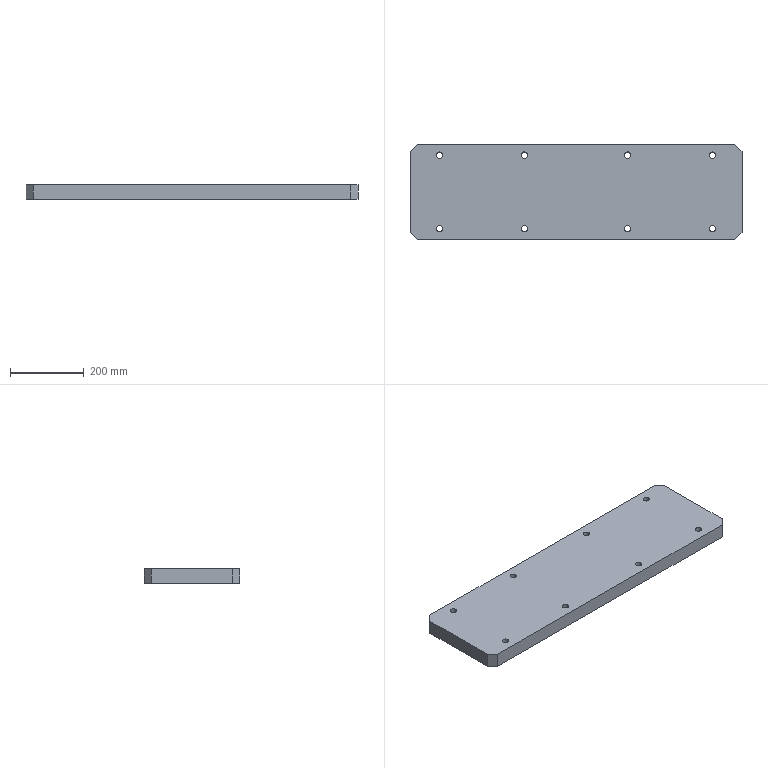Part | SolidWorks | features Chamfer 1, Extrusion 1, HoleWzd 1 | 1 solid | 26 faces | box 900 x 260 x 40 mm | volume 9255366 mm3 | cylinder 16 | plane 10 | commonest cylinder face diameters 17 x16
STEP:
#1=CARTESIAN_POINT('',(-378.5,100.,0.));
#2=VERTEX_POINT('',#1);
#3=CARTESIAN_POINT('',(-361.5,100.,0.));
#4=VERTEX_POINT('',#3);
#5=CARTESIAN_POINT('',(-370.,100.,0.));
#6=DIRECTION('',(0.,0.,1.));
#7=DIRECTION('',(1.,0.,0.));
#8=AXIS2_PLACEMENT_3D('',#5,#6,#7);
#9=CIRCLE('',#8,8.5);
#10=EDGE_CURVE('',#2,#4,#9,.T.);
#11=ORIENTED_EDGE('',*,*,#10,.F.);
#12=CARTESIAN_POINT('',(-378.5,100.,40.));
#13=VERTEX_POINT('',#12);
#14=CARTESIAN_POINT('',(-378.5,100.,40.));
#15=DIRECTION('',(0.,0.,1.));
#16=VECTOR('',#15,1000.);
#17=LINE('',#14,#16);
#18=EDGE_CURVE('',#2,#13,#17,.T.);
#19=ORIENTED_EDGE('',*,*,#18,.T.);
#20=CARTESIAN_POINT('',(-361.5,100.,40.));
#21=VERTEX_POINT('',#20);
#22=CARTESIAN_POINT('',(-370.,100.,40.));
#23=DIRECTION('',(0.,0.,1.));
#24=DIRECTION('',(1.,0.,0.));
#25=AXIS2_PLACEMENT_3D('',#22,#23,#24);
#26=CIRCLE('',#25,8.5);
#27=EDGE_CURVE('',#13,#21,#26,.T.);
#28=ORIENTED_EDGE('',*,*,#27,.T.);
#29=CARTESIAN_POINT('',(-361.5,100.,40.));
#30=DIRECTION('',(0.,0.,1.));
#31=VECTOR('',#30,1000.);
#32=LINE('',#29,#31);
#33=EDGE_CURVE('',#4,#21,#32,.T.);
#34=ORIENTED_EDGE('',*,*,#33,.F.);
#35=EDGE_LOOP('',(#11,#19,#28,#34));
#36=FACE_OUTER_BOUND('',#35,.T.);
#37=CARTESIAN_POINT('',(-370.,100.,40.));
#38=DIRECTION('',(0.,0.,1.));
#39=DIRECTION('',(1.,0.,0.));
#40=AXIS2_PLACEMENT_3D('',#37,#38,#39);
#41=CYLINDRICAL_SURFACE('',#40,8.5);
#42=ADVANCED_FACE('',(#36),#41,.F.);
#43=CARTESIAN_POINT('',(-148.5,100.,0.));
#44=VERTEX_POINT('',#43);
#45=CARTESIAN_POINT('',(-131.5,100.,0.));
#46=VERTEX_POINT('',#45);
#47=CARTESIAN_POINT('',(-140.,100.,0.));
#48=DIRECTION('',(0.,0.,1.));
#49=DIRECTION('',(1.,0.,0.));
#50=AXIS2_PLACEMENT_3D('',#47,#48,#49);
#51=CIRCLE('',#50,8.5);
#52=EDGE_CURVE('',#44,#46,#51,.T.);
#53=ORIENTED_EDGE('',*,*,#52,.F.);
#54=CARTESIAN_POINT('',(-148.5,100.,40.));
#55=VERTEX_POINT('',#54);
#56=CARTESIAN_POINT('',(-148.5,100.,40.));
#57=DIRECTION('',(0.,0.,1.));
#58=VECTOR('',#57,1000.);
#59=LINE('',#56,#58);
#60=EDGE_CURVE('',#44,#55,#59,.T.);
#61=ORIENTED_EDGE('',*,*,#60,.T.);
#62=CARTESIAN_POINT('',(-131.5,100.,40.));
#63=VERTEX_POINT('',#62);
#64=CARTESIAN_POINT('',(-140.,100.,40.));
#65=DIRECTION('',(0.,0.,1.));
#66=DIRECTION('',(1.,0.,0.));
#67=AXIS2_PLACEMENT_3D('',#64,#65,#66);
#68=CIRCLE('',#67,8.5);
#69=EDGE_CURVE('',#55,#63,#68,.T.);
#70=ORIENTED_EDGE('',*,*,#69,.T.);
#71=CARTESIAN_POINT('',(-131.5,100.,40.));
#72=DIRECTION('',(0.,0.,1.));
#73=VECTOR('',#72,1000.);
#74=LINE('',#71,#73);
#75=EDGE_CURVE('',#46,#63,#74,.T.);
#76=ORIENTED_EDGE('',*,*,#75,.F.);
#77=EDGE_LOOP('',(#53,#61,#70,#76));
#78=FACE_OUTER_BOUND('',#77,.T.);
#79=CARTESIAN_POINT('',(-140.,100.,40.));
#80=DIRECTION('',(0.,0.,1.));
#81=DIRECTION('',(1.,0.,0.));
#82=AXIS2_PLACEMENT_3D('',#79,#80,#81);
#83=CYLINDRICAL_SURFACE('',#82,8.5);
#84=ADVANCED_FACE('',(#78),#83,.F.);
#85=CARTESIAN_POINT('',(-378.5,-100.,0.));
#86=VERTEX_POINT('',#85);
#87=CARTESIAN_POINT('',(-361.5,-100.,0.));
#88=VERTEX_POINT('',#87);
#89=CARTESIAN_POINT('',(-370.,-100.,0.));
#90=DIRECTION('',(0.,0.,1.));
#91=DIRECTION('',(1.,0.,0.));
#92=AXIS2_PLACEMENT_3D('',#89,#90,#91);
#93=CIRCLE('',#92,8.5);
#94=EDGE_CURVE('',#86,#88,#93,.T.);
#95=ORIENTED_EDGE('',*,*,#94,.F.);
#96=CARTESIAN_POINT('',(-378.5,-100.,40.));
#97=VERTEX_POINT('',#96);
#98=CARTESIAN_POINT('',(-378.5,-100.,40.));
#99=DIRECTION('',(0.,0.,1.));
#100=VECTOR('',#99,1000.);
#101=LINE('',#98,#100);
#102=EDGE_CURVE('',#86,#97,#101,.T.);
#103=ORIENTED_EDGE('',*,*,#102,.T.);
#104=CARTESIAN_POINT('',(-361.5,-100.,40.));
#105=VERTEX_POINT('',#104);
#106=CARTESIAN_POINT('',(-370.,-100.,40.));
#107=DIRECTION('',(0.,0.,1.));
#108=DIRECTION('',(1.,0.,0.));
#109=AXIS2_PLACEMENT_3D('',#106,#107,#108);
#110=CIRCLE('',#109,8.5);
#111=EDGE_CURVE('',#97,#105,#110,.T.);
#112=ORIENTED_EDGE('',*,*,#111,.T.);
#113=CARTESIAN_POINT('',(-361.5,-100.,40.));
#114=DIRECTION('',(0.,0.,1.));
#115=VECTOR('',#114,1000.);
#116=LINE('',#113,#115);
#117=EDGE_CURVE('',#88,#105,#116,.T.);
#118=ORIENTED_EDGE('',*,*,#117,.F.);
#119=EDGE_LOOP('',(#95,#103,#112,#118));
#120=FACE_OUTER_BOUND('',#119,.T.);
#121=CARTESIAN_POINT('',(-370.,-100.,40.));
#122=DIRECTION('',(0.,0.,1.));
#123=DIRECTION('',(1.,0.,0.));
#124=AXIS2_PLACEMENT_3D('',#121,#122,#123);
#125=CYLINDRICAL_SURFACE('',#124,8.5);
#126=ADVANCED_FACE('',(#120),#125,.F.);
#127=CARTESIAN_POINT('',(-148.5,-100.,0.));
#128=VERTEX_POINT('',#127);
#129=CARTESIAN_POINT('',(-131.5,-100.,0.));
#130=VERTEX_POINT('',#129);
#131=CARTESIAN_POINT('',(-140.,-100.,0.));
#132=DIRECTION('',(0.,0.,1.));
#133=DIRECTION('',(1.,0.,0.));
#134=AXIS2_PLACEMENT_3D('',#131,#132,#133);
#135=CIRCLE('',#134,8.5);
#136=EDGE_CURVE('',#128,#130,#135,.T.);
#137=ORIENTED_EDGE('',*,*,#136,.F.);
#138=CARTESIAN_POINT('',(-148.5,-100.,40.));
#139=VERTEX_POINT('',#138);
#140=CARTESIAN_POINT('',(-148.5,-100.,40.));
#141=DIRECTION('',(0.,0.,1.));
#142=VECTOR('',#141,1000.);
#143=LINE('',#140,#142);
#144=EDGE_CURVE('',#128,#139,#143,.T.);
#145=ORIENTED_EDGE('',*,*,#144,.T.);
#146=CARTESIAN_POINT('',(-131.5,-100.,40.));
#147=VERTEX_POINT('',#146);
#148=CARTESIAN_POINT('',(-140.,-100.,40.));
#149=DIRECTION('',(0.,0.,1.));
#150=DIRECTION('',(1.,0.,0.));
#151=AXIS2_PLACEMENT_3D('',#148,#149,#150);
#152=CIRCLE('',#151,8.5);
#153=EDGE_CURVE('',#139,#147,#152,.T.);
#154=ORIENTED_EDGE('',*,*,#153,.T.);
#155=CARTESIAN_POINT('',(-131.5,-100.,40.));
#156=DIRECTION('',(0.,0.,1.));
#157=VECTOR('',#156,1000.);
#158=LINE('',#155,#157);
#159=EDGE_CURVE('',#130,#147,#158,.T.);
#160=ORIENTED_EDGE('',*,*,#159,.F.);
#161=EDGE_LOOP('',(#137,#145,#154,#160));
#162=FACE_OUTER_BOUND('',#161,.T.);
#163=CARTESIAN_POINT('',(-140.,-100.,40.));
#164=DIRECTION('',(0.,0.,1.));
#165=DIRECTION('',(1.,0.,0.));
#166=AXIS2_PLACEMENT_3D('',#163,#164,#165);
#167=CYLINDRICAL_SURFACE('',#166,8.5);
#168=ADVANCED_FACE('',(#162),#167,.F.);
#169=CARTESIAN_POINT('',(131.5,-100.,0.));
#170=VERTEX_POINT('',#169);
#171=CARTESIAN_POINT('',(148.5,-100.,0.));
#172=VERTEX_POINT('',#171);
#173=CARTESIAN_POINT('',(140.,-100.,0.));
#174=DIRECTION('',(0.,0.,1.));
#175=DIRECTION('',(1.,0.,0.));
#176=AXIS2_PLACEMENT_3D('',#173,#174,#175);
#177=CIRCLE('',#176,8.5);
#178=EDGE_CURVE('',#170,#172,#177,.T.);
#179=ORIENTED_EDGE('',*,*,#178,.F.);
#180=CARTESIAN_POINT('',(131.5,-100.,40.));
#181=VERTEX_POINT('',#180);
#182=CARTESIAN_POINT('',(131.5,-100.,40.));
#183=DIRECTION('',(0.,0.,1.));
#184=VECTOR('',#183,1000.);
#185=LINE('',#182,#184);
#186=EDGE_CURVE('',#170,#181,#185,.T.);
#187=ORIENTED_EDGE('',*,*,#186,.T.);
#188=CARTESIAN_POINT('',(148.5,-100.,40.));
#189=VERTEX_POINT('',#188);
#190=CARTESIAN_POINT('',(140.,-100.,40.));
#191=DIRECTION('',(0.,0.,1.));
#192=DIRECTION('',(1.,0.,0.));
#193=AXIS2_PLACEMENT_3D('',#190,#191,#192);
#194=CIRCLE('',#193,8.5);
#195=EDGE_CURVE('',#181,#189,#194,.T.);
#196=ORIENTED_EDGE('',*,*,#195,.T.);
#197=CARTESIAN_POINT('',(148.5,-100.,40.));
#198=DIRECTION('',(0.,0.,1.));
#199=VECTOR('',#198,1000.);
#200=LINE('',#197,#199);
#201=EDGE_CURVE('',#172,#189,#200,.T.);
#202=ORIENTED_EDGE('',*,*,#201,.F.);
#203=EDGE_LOOP('',(#179,#187,#196,#202));
#204=FACE_OUTER_BOUND('',#203,.T.);
#205=CARTESIAN_POINT('',(140.,-100.,40.));
#206=DIRECTION('',(0.,0.,1.));
#207=DIRECTION('',(1.,0.,0.));
#208=AXIS2_PLACEMENT_3D('',#205,#206,#207);
#209=CYLINDRICAL_SURFACE('',#208,8.5);
#210=ADVANCED_FACE('',(#204),#209,.F.);
#211=CARTESIAN_POINT('',(361.5,-100.,0.));
#212=VERTEX_POINT('',#211);
#213=CARTESIAN_POINT('',(378.5,-100.,0.));
#214=VERTEX_POINT('',#213);
#215=CARTESIAN_POINT('',(370.,-100.,0.));
#216=DIRECTION('',(0.,0.,1.));
#217=DIRECTION('',(1.,0.,0.));
#218=AXIS2_PLACEMENT_3D('',#215,#216,#217);
#219=CIRCLE('',#218,8.5);
#220=EDGE_CURVE('',#212,#214,#219,.T.);
#221=ORIENTED_EDGE('',*,*,#220,.F.);
#222=CARTESIAN_POINT('',(361.5,-100.,40.));
#223=VERTEX_POINT('',#222);
#224=CARTESIAN_POINT('',(361.5,-100.,40.));
#225=DIRECTION('',(0.,0.,1.));
#226=VECTOR('',#225,1000.);
#227=LINE('',#224,#226);
#228=EDGE_CURVE('',#212,#223,#227,.T.);
#229=ORIENTED_EDGE('',*,*,#228,.T.);
#230=CARTESIAN_POINT('',(378.5,-100.,40.));
#231=VERTEX_POINT('',#230);
#232=CARTESIAN_POINT('',(370.,-100.,40.));
#233=DIRECTION('',(0.,0.,1.));
#234=DIRECTION('',(1.,0.,0.));
#235=AXIS2_PLACEMENT_3D('',#232,#233,#234);
#236=CIRCLE('',#235,8.5);
#237=EDGE_CURVE('',#223,#231,#236,.T.);
#238=ORIENTED_EDGE('',*,*,#237,.T.);
#239=CARTESIAN_POINT('',(378.5,-100.,40.));
#240=DIRECTION('',(0.,0.,1.));
#241=VECTOR('',#240,1000.);
#242=LINE('',#239,#241);
#243=EDGE_CURVE('',#214,#231,#242,.T.);
#244=ORIENTED_EDGE('',*,*,#243,.F.);
#245=EDGE_LOOP('',(#221,#229,#238,#244));
#246=FACE_OUTER_BOUND('',#245,.T.);
#247=CARTESIAN_POINT('',(370.,-100.,40.));
#248=DIRECTION('',(0.,0.,1.));
#249=DIRECTION('',(1.,0.,0.));
#250=AXIS2_PLACEMENT_3D('',#247,#248,#249);
#251=CYLINDRICAL_SURFACE('',#250,8.5);
#252=ADVANCED_FACE('',(#246),#251,.F.);
#253=CARTESIAN_POINT('',(131.5,100.,0.));
#254=VERTEX_POINT('',#253);
#255=CARTESIAN_POINT('',(148.5,100.,0.));
#256=VERTEX_POINT('',#255);
#257=CARTESIAN_POINT('',(140.,100.,0.));
#258=DIRECTION('',(0.,0.,1.));
#259=DIRECTION('',(1.,0.,0.));
#260=AXIS2_PLACEMENT_3D('',#257,#258,#259);
#261=CIRCLE('',#260,8.5);
#262=EDGE_CURVE('',#254,#256,#261,.T.);
#263=ORIENTED_EDGE('',*,*,#262,.F.);
#264=CARTESIAN_POINT('',(131.5,100.,40.));
#265=VERTEX_POINT('',#264);
#266=CARTESIAN_POINT('',(131.5,100.,40.));
#267=DIRECTION('',(0.,0.,1.));
#268=VECTOR('',#267,1000.);
#269=LINE('',#266,#268);
#270=EDGE_CURVE('',#254,#265,#269,.T.);
#271=ORIENTED_EDGE('',*,*,#270,.T.);
#272=CARTESIAN_POINT('',(148.5,100.,40.));
#273=VERTEX_POINT('',#272);
#274=CARTESIAN_POINT('',(140.,100.,40.));
#275=DIRECTION('',(0.,0.,1.));
#276=DIRECTION('',(1.,0.,0.));
#277=AXIS2_PLACEMENT_3D('',#274,#275,#276);
#278=CIRCLE('',#277,8.5);
#279=EDGE_CURVE('',#265,#273,#278,.T.);
#280=ORIENTED_EDGE('',*,*,#279,.T.);
#281=CARTESIAN_POINT('',(148.5,100.,40.));
#282=DIRECTION('',(0.,0.,1.));
#283=VECTOR('',#282,1000.);
#284=LINE('',#281,#283);
#285=EDGE_CURVE('',#256,#273,#284,.T.);
#286=ORIENTED_EDGE('',*,*,#285,.F.);
#287=EDGE_LOOP('',(#263,#271,#280,#286));
#288=FACE_OUTER_BOUND('',#287,.T.);
#289=CARTESIAN_POINT('',(140.,100.,40.));
#290=DIRECTION('',(0.,0.,1.));
#291=DIRECTION('',(1.,0.,0.));
#292=AXIS2_PLACEMENT_3D('',#289,#290,#291);
#293=CYLINDRICAL_SURFACE('',#292,8.5);
#294=ADVANCED_FACE('',(#288),#293,.F.);
#295=CARTESIAN_POINT('',(361.5,100.,0.));
#296=VERTEX_POINT('',#295);
#297=CARTESIAN_POINT('',(378.5,100.,0.));
#298=VERTEX_POINT('',#297);
#299=CARTESIAN_POINT('',(370.,100.,0.));
#300=DIRECTION('',(0.,0.,1.));
#301=DIRECTION('',(1.,0.,0.));
#302=AXIS2_PLACEMENT_3D('',#299,#300,#301);
#303=CIRCLE('',#302,8.5);
#304=EDGE_CURVE('',#296,#298,#303,.T.);
#305=ORIENTED_EDGE('',*,*,#304,.F.);
#306=CARTESIAN_POINT('',(361.5,100.,40.));
#307=VERTEX_POINT('',#306);
#308=CARTESIAN_POINT('',(361.5,100.,40.));
#309=DIRECTION('',(0.,0.,1.));
#310=VECTOR('',#309,1000.);
#311=LINE('',#308,#310);
#312=EDGE_CURVE('',#296,#307,#311,.T.);
#313=ORIENTED_EDGE('',*,*,#312,.T.);
#314=CARTESIAN_POINT('',(378.5,100.,40.));
#315=VERTEX_POINT('',#314);
#316=CARTESIAN_POINT('',(370.,100.,40.));
#317=DIRECTION('',(0.,0.,1.));
#318=DIRECTION('',(1.,0.,0.));
#319=AXIS2_PLACEMENT_3D('',#316,#317,#318);
#320=CIRCLE('',#319,8.5);
#321=EDGE_CURVE('',#307,#315,#320,.T.);
#322=ORIENTED_EDGE('',*,*,#321,.T.);
#323=CARTESIAN_POINT('',(378.5,100.,40.));
#324=DIRECTION('',(0.,0.,1.));
#325=VECTOR('',#324,1000.);
#326=LINE('',#323,#325);
#327=EDGE_CURVE('',#298,#315,#326,.T.);
#328=ORIENTED_EDGE('',*,*,#327,.F.);
#329=EDGE_LOOP('',(#305,#313,#322,#328));
#330=FACE_OUTER_BOUND('',#329,.T.);
#331=CARTESIAN_POINT('',(370.,100.,40.));
#332=DIRECTION('',(0.,0.,1.));
#333=DIRECTION('',(1.,0.,0.));
#334=AXIS2_PLACEMENT_3D('',#331,#332,#333);
#335=CYLINDRICAL_SURFACE('',#334,8.5);
#336=ADVANCED_FACE('',(#330),#335,.F.);
#337=CARTESIAN_POINT('',(-450.,110.,40.));
#338=VERTEX_POINT('',#337);
#339=CARTESIAN_POINT('',(-450.,-110.,40.));
#340=VERTEX_POINT('',#339);
#341=CARTESIAN_POINT('',(-450.,-130.,40.));
#342=DIRECTION('',(0.,-1.,0.));
#343=VECTOR('',#342,1000.);
#344=LINE('',#341,#343);
#345=EDGE_CURVE('',#338,#340,#344,.T.);
#346=ORIENTED_EDGE('',*,*,#345,.F.);
#347=CARTESIAN_POINT('',(-450.,110.,0.));
#348=VERTEX_POINT('',#347);
#349=CARTESIAN_POINT('',(-450.,110.,40.));
#350=DIRECTION('',(0.,0.,-1.));
#351=VECTOR('',#350,1000.);
#352=LINE('',#349,#351);
#353=EDGE_CURVE('',#338,#348,#352,.T.);
#354=ORIENTED_EDGE('',*,*,#353,.T.);
#355=CARTESIAN_POINT('',(-450.,-110.,0.));
#356=VERTEX_POINT('',#355);
#357=CARTESIAN_POINT('',(-450.,-130.,0.));
#358=DIRECTION('',(0.,-1.,0.));
#359=VECTOR('',#358,1000.);
#360=LINE('',#357,#359);
#361=EDGE_CURVE('',#348,#356,#360,.T.);
#362=ORIENTED_EDGE('',*,*,#361,.T.);
#363=CARTESIAN_POINT('',(-450.,-110.,40.));
#364=DIRECTION('',(0.,0.,1.));
#365=VECTOR('',#364,1000.);
#366=LINE('',#363,#365);
#367=EDGE_CURVE('',#356,#340,#366,.T.);
#368=ORIENTED_EDGE('',*,*,#367,.T.);
#369=EDGE_LOOP('',(#346,#354,#362,#368));
#370=FACE_OUTER_BOUND('',#369,.T.);
#371=CARTESIAN_POINT('',(-450.,-130.,40.));
#372=DIRECTION('',(1.,0.,0.));
#373=DIRECTION('',(0.,0.,-1.));
#374=AXIS2_PLACEMENT_3D('',#371,#372,#373);
#375=PLANE('',#374);
#376=ADVANCED_FACE('',(#370),#375,.F.);
#377=CARTESIAN_POINT('',(-430.,-130.,0.));
#378=VERTEX_POINT('',#377);
#379=CARTESIAN_POINT('',(430.,-130.,0.));
#380=VERTEX_POINT('',#379);
#381=CARTESIAN_POINT('',(450.,-130.,0.));
#382=DIRECTION('',(1.,0.,0.));
#383=VECTOR('',#382,1000.);
#384=LINE('',#381,#383);
#385=EDGE_CURVE('',#378,#380,#384,.T.);
#386=ORIENTED_EDGE('',*,*,#385,.T.);
#387=CARTESIAN_POINT('',(430.,-130.,40.));
#388=VERTEX_POINT('',#387);
#389=CARTESIAN_POINT('',(430.,-130.,40.));
#390=DIRECTION('',(0.,0.,1.));
#391=VECTOR('',#390,1000.);
#392=LINE('',#389,#391);
#393=EDGE_CURVE('',#380,#388,#392,.T.);
#394=ORIENTED_EDGE('',*,*,#393,.T.);
#395=CARTESIAN_POINT('',(-430.,-130.,40.));
#396=VERTEX_POINT('',#395);
#397=CARTESIAN_POINT('',(450.,-130.,40.));
#398=DIRECTION('',(1.,0.,0.));
#399=VECTOR('',#398,1000.);
#400=LINE('',#397,#399);
#401=EDGE_CURVE('',#396,#388,#400,.T.);
#402=ORIENTED_EDGE('',*,*,#401,.F.);
#403=CARTESIAN_POINT('',(-430.,-130.,40.));
#404=DIRECTION('',(0.,0.,-1.));
#405=VECTOR('',#404,1000.);
#406=LINE('',#403,#405);
#407=EDGE_CURVE('',#396,#378,#406,.T.);
#408=ORIENTED_EDGE('',*,*,#407,.T.);
#409=EDGE_LOOP('',(#386,#394,#402,#408));
#410=FACE_OUTER_BOUND('',#409,.T.);
#411=CARTESIAN_POINT('',(450.,-130.,40.));
#412=DIRECTION('',(0.,1.,0.));
#413=DIRECTION('',(-1.,0.,0.));
#414=AXIS2_PLACEMENT_3D('',#411,#412,#413);
#415=PLANE('',#414);
#416=ADVANCED_FACE('',(#410),#415,.F.);
#417=CARTESIAN_POINT('',(450.,-110.,0.));
#418=VERTEX_POINT('',#417);
#419=CARTESIAN_POINT('',(450.,110.,0.));
#420=VERTEX_POINT('',#419);
#421=CARTESIAN_POINT('',(450.,-130.,0.));
#422=DIRECTION('',(0.,1.,0.));
#423=VECTOR('',#422,1000.);
#424=LINE('',#421,#423);
#425=EDGE_CURVE('',#418,#420,#424,.T.);
#426=ORIENTED_EDGE('',*,*,#425,.T.);
#427=CARTESIAN_POINT('',(450.,110.,40.));
#428=VERTEX_POINT('',#427);
#429=CARTESIAN_POINT('',(450.,110.,40.));
#430=DIRECTION('',(0.,0.,1.));
#431=VECTOR('',#430,1000.);
#432=LINE('',#429,#431);
#433=EDGE_CURVE('',#420,#428,#432,.T.);
#434=ORIENTED_EDGE('',*,*,#433,.T.);
#435=CARTESIAN_POINT('',(450.,-110.,40.));
#436=VERTEX_POINT('',#435);
#437=CARTESIAN_POINT('',(450.,-130.,40.));
#438=DIRECTION('',(0.,1.,0.));
#439=VECTOR('',#438,1000.);
#440=LINE('',#437,#439);
#441=EDGE_CURVE('',#436,#428,#440,.T.);
#442=ORIENTED_EDGE('',*,*,#441,.F.);
#443=CARTESIAN_POINT('',(450.,-110.,40.));
#444=DIRECTION('',(0.,0.,-1.));
#445=VECTOR('',#444,1000.);
#446=LINE('',#443,#445);
#447=EDGE_CURVE('',#436,#418,#446,.T.);
#448=ORIENTED_EDGE('',*,*,#447,.T.);
#449=EDGE_LOOP('',(#426,#434,#442,#448));
#450=FACE_OUTER_BOUND('',#449,.T.);
#451=CARTESIAN_POINT('',(450.,-130.,40.));
#452=DIRECTION('',(-1.,0.,0.));
#453=DIRECTION('',(0.,0.,1.));
#454=AXIS2_PLACEMENT_3D('',#451,#452,#453);
#455=PLANE('',#454);
#456=ADVANCED_FACE('',(#450),#455,.F.);
#457=CARTESIAN_POINT('',(430.,130.,0.));
#458=VERTEX_POINT('',#457);
#459=CARTESIAN_POINT('',(-430.,130.,0.));
#460=VERTEX_POINT('',#459);
#461=CARTESIAN_POINT('',(450.,130.,0.));
#462=DIRECTION('',(-1.,0.,0.));
#463=VECTOR('',#462,1000.);
#464=LINE('',#461,#463);
#465=EDGE_CURVE('',#458,#460,#464,.T.);
#466=ORIENTED_EDGE('',*,*,#465,.T.);
#467=CARTESIAN_POINT('',(-430.,130.,40.));
#468=VERTEX_POINT('',#467);
#469=CARTESIAN_POINT('',(-430.,130.,40.));
#470=DIRECTION('',(0.,0.,1.));
#471=VECTOR('',#470,1000.);
#472=LINE('',#469,#471);
#473=EDGE_CURVE('',#460,#468,#472,.T.);
#474=ORIENTED_EDGE('',*,*,#473,.T.);
#475=CARTESIAN_POINT('',(430.,130.,40.));
#476=VERTEX_POINT('',#475);
#477=CARTESIAN_POINT('',(450.,130.,40.));
#478=DIRECTION('',(-1.,0.,0.));
#479=VECTOR('',#478,1000.);
#480=LINE('',#477,#479);
#481=EDGE_CURVE('',#476,#468,#480,.T.);
#482=ORIENTED_EDGE('',*,*,#481,.F.);
#483=CARTESIAN_POINT('',(430.,130.,40.));
#484=DIRECTION('',(0.,0.,-1.));
#485=VECTOR('',#484,1000.);
#486=LINE('',#483,#485);
#487=EDGE_CURVE('',#476,#458,#486,.T.);
#488=ORIENTED_EDGE('',*,*,#487,.T.);
#489=EDGE_LOOP('',(#466,#474,#482,#488));
#490=FACE_OUTER_BOUND('',#489,.T.);
#491=CARTESIAN_POINT('',(450.,130.,40.));
#492=DIRECTION('',(0.,-1.,0.));
#493=DIRECTION('',(1.,0.,0.));
#494=AXIS2_PLACEMENT_3D('',#491,#492,#493);
#495=PLANE('',#494);
#496=ADVANCED_FACE('',(#490),#495,.F.);
#497=CARTESIAN_POINT('',(-370.,100.,40.));
#498=DIRECTION('',(0.,0.,1.));
#499=DIRECTION('',(1.,0.,0.));
#500=AXIS2_PLACEMENT_3D('',#497,#498,#499);
#501=CIRCLE('',#500,8.5);
#502=EDGE_CURVE('',#21,#13,#501,.T.);
#503=ORIENTED_EDGE('',*,*,#502,.F.);
#504=ORIENTED_EDGE('',*,*,#27,.F.);
#505=EDGE_LOOP('',(#503,#504));
#506=FACE_BOUND('',#505,.T.);
#507=CARTESIAN_POINT('',(-140.,100.,40.));
#508=DIRECTION('',(0.,0.,1.));
#509=DIRECTION('',(1.,0.,0.));
#510=AXIS2_PLACEMENT_3D('',#507,#508,#509);
#511=CIRCLE('',#510,8.5);
#512=EDGE_CURVE('',#63,#55,#511,.T.);
#513=ORIENTED_EDGE('',*,*,#512,.F.);
#514=ORIENTED_EDGE('',*,*,#69,.F.);
#515=EDGE_LOOP('',(#513,#514));
#516=FACE_BOUND('',#515,.T.);
#517=CARTESIAN_POINT('',(-370.,-100.,40.));
#518=DIRECTION('',(0.,0.,1.));
#519=DIRECTION('',(1.,0.,0.));
#520=AXIS2_PLACEMENT_3D('',#517,#518,#519);
#521=CIRCLE('',#520,8.5);
#522=EDGE_CURVE('',#105,#97,#521,.T.);
#523=ORIENTED_EDGE('',*,*,#522,.F.);
#524=ORIENTED_EDGE('',*,*,#111,.F.);
#525=EDGE_LOOP('',(#523,#524));
#526=FACE_BOUND('',#525,.T.);
#527=CARTESIAN_POINT('',(-140.,-100.,40.));
#528=DIRECTION('',(0.,0.,1.));
#529=DIRECTION('',(1.,0.,0.));
#530=AXIS2_PLACEMENT_3D('',#527,#528,#529);
#531=CIRCLE('',#530,8.5);
#532=EDGE_CURVE('',#147,#139,#531,.T.);
#533=ORIENTED_EDGE('',*,*,#532,.F.);
#534=ORIENTED_EDGE('',*,*,#153,.F.);
#535=EDGE_LOOP('',(#533,#534));
#536=FACE_BOUND('',#535,.T.);
#537=CARTESIAN_POINT('',(140.,-100.,40.));
#538=DIRECTION('',(0.,0.,1.));
#539=DIRECTION('',(1.,0.,0.));
#540=AXIS2_PLACEMENT_3D('',#537,#538,#539);
#541=CIRCLE('',#540,8.5);
#542=EDGE_CURVE('',#189,#181,#541,.T.);
#543=ORIENTED_EDGE('',*,*,#542,.F.);
#544=ORIENTED_EDGE('',*,*,#195,.F.);
#545=EDGE_LOOP('',(#543,#544));
#546=FACE_BOUND('',#545,.T.);
#547=CARTESIAN_POINT('',(370.,-100.,40.));
#548=DIRECTION('',(0.,0.,1.));
#549=DIRECTION('',(1.,0.,0.));
#550=AXIS2_PLACEMENT_3D('',#547,#548,#549);
#551=CIRCLE('',#550,8.5);
#552=EDGE_CURVE('',#231,#223,#551,.T.);
#553=ORIENTED_EDGE('',*,*,#552,.F.);
#554=ORIENTED_EDGE('',*,*,#237,.F.);
#555=EDGE_LOOP('',(#553,#554));
#556=FACE_BOUND('',#555,.T.);
#557=CARTESIAN_POINT('',(140.,100.,40.));
#558=DIRECTION('',(0.,0.,1.));
#559=DIRECTION('',(1.,0.,0.));
#560=AXIS2_PLACEMENT_3D('',#557,#558,#559);
#561=CIRCLE('',#560,8.5);
#562=EDGE_CURVE('',#273,#265,#561,.T.);
#563=ORIENTED_EDGE('',*,*,#562,.F.);
#564=ORIENTED_EDGE('',*,*,#279,.F.);
#565=EDGE_LOOP('',(#563,#564));
#566=FACE_BOUND('',#565,.T.);
#567=CARTESIAN_POINT('',(370.,100.,40.));
#568=DIRECTION('',(0.,0.,1.));
#569=DIRECTION('',(1.,0.,0.));
#570=AXIS2_PLACEMENT_3D('',#567,#568,#569);
#571=CIRCLE('',#570,8.5);
#572=EDGE_CURVE('',#315,#307,#571,.T.);
#573=ORIENTED_EDGE('',*,*,#572,.F.);
#574=ORIENTED_EDGE('',*,*,#321,.F.);
#575=EDGE_LOOP('',(#573,#574));
#576=FACE_BOUND('',#575,.T.);
#577=ORIENTED_EDGE('',*,*,#481,.T.);
#578=CARTESIAN_POINT('',(-280.,280.,40.));
#579=DIRECTION('',(-0.7071,-0.7071,0.));
#580=VECTOR('',#579,1000.);
#581=LINE('',#578,#580);
#582=EDGE_CURVE('',#468,#338,#581,.T.);
#583=ORIENTED_EDGE('',*,*,#582,.T.);
#584=ORIENTED_EDGE('',*,*,#345,.T.);
#585=CARTESIAN_POINT('',(-280.,-280.,40.));
#586=DIRECTION('',(0.7071,-0.7071,0.));
#587=VECTOR('',#586,1000.);
#588=LINE('',#585,#587);
#589=EDGE_CURVE('',#340,#396,#588,.T.);
#590=ORIENTED_EDGE('',*,*,#589,.T.);
#591=ORIENTED_EDGE('',*,*,#401,.T.);
#592=CARTESIAN_POINT('',(280.,-280.,40.));
#593=DIRECTION('',(0.7071,0.7071,0.));
#594=VECTOR('',#593,1000.);
#595=LINE('',#592,#594);
#596=EDGE_CURVE('',#388,#436,#595,.T.);
#597=ORIENTED_EDGE('',*,*,#596,.T.);
#598=ORIENTED_EDGE('',*,*,#441,.T.);
#599=CARTESIAN_POINT('',(280.,280.,40.));
#600=DIRECTION('',(-0.7071,0.7071,0.));
#601=VECTOR('',#600,1000.);
#602=LINE('',#599,#601);
#603=EDGE_CURVE('',#428,#476,#602,.T.);
#604=ORIENTED_EDGE('',*,*,#603,.T.);
#605=EDGE_LOOP('',(#577,#583,#584,#590,#591,#597,#598,#604));
#606=FACE_OUTER_BOUND('',#605,.T.);
#607=CARTESIAN_POINT('',(0.,0.,40.));
#608=DIRECTION('',(0.,0.,1.));
#609=DIRECTION('',(1.,0.,0.));
#610=AXIS2_PLACEMENT_3D('',#607,#608,#609);
#611=PLANE('',#610);
#612=ADVANCED_FACE('',(#506,#516,#526,#536,#546,#556,#566,#576,#606),#611,.T.);
#613=CARTESIAN_POINT('',(-370.,100.,0.));
#614=DIRECTION('',(0.,0.,1.));
#615=DIRECTION('',(1.,0.,0.));
#616=AXIS2_PLACEMENT_3D('',#613,#614,#615);
#617=CIRCLE('',#616,8.5);
#618=EDGE_CURVE('',#4,#2,#617,.T.);
#619=ORIENTED_EDGE('',*,*,#618,.T.);
#620=ORIENTED_EDGE('',*,*,#10,.T.);
#621=EDGE_LOOP('',(#619,#620));
#622=FACE_BOUND('',#621,.T.);
#623=CARTESIAN_POINT('',(-140.,100.,0.));
#624=DIRECTION('',(0.,0.,1.));
#625=DIRECTION('',(1.,0.,0.));
#626=AXIS2_PLACEMENT_3D('',#623,#624,#625);
#627=CIRCLE('',#626,8.5);
#628=EDGE_CURVE('',#46,#44,#627,.T.);
#629=ORIENTED_EDGE('',*,*,#628,.T.);
#630=ORIENTED_EDGE('',*,*,#52,.T.);
#631=EDGE_LOOP('',(#629,#630));
#632=FACE_BOUND('',#631,.T.);
#633=CARTESIAN_POINT('',(-370.,-100.,0.));
#634=DIRECTION('',(0.,0.,1.));
#635=DIRECTION('',(1.,0.,0.));
#636=AXIS2_PLACEMENT_3D('',#633,#634,#635);
#637=CIRCLE('',#636,8.5);
#638=EDGE_CURVE('',#88,#86,#637,.T.);
#639=ORIENTED_EDGE('',*,*,#638,.T.);
#640=ORIENTED_EDGE('',*,*,#94,.T.);
#641=EDGE_LOOP('',(#639,#640));
#642=FACE_BOUND('',#641,.T.);
#643=CARTESIAN_POINT('',(-140.,-100.,0.));
#644=DIRECTION('',(0.,0.,1.));
#645=DIRECTION('',(1.,0.,0.));
#646=AXIS2_PLACEMENT_3D('',#643,#644,#645);
#647=CIRCLE('',#646,8.5);
#648=EDGE_CURVE('',#130,#128,#647,.T.);
#649=ORIENTED_EDGE('',*,*,#648,.T.);
#650=ORIENTED_EDGE('',*,*,#136,.T.);
#651=EDGE_LOOP('',(#649,#650));
#652=FACE_BOUND('',#651,.T.);
#653=CARTESIAN_POINT('',(140.,-100.,0.));
#654=DIRECTION('',(0.,0.,1.));
#655=DIRECTION('',(1.,0.,0.));
#656=AXIS2_PLACEMENT_3D('',#653,#654,#655);
#657=CIRCLE('',#656,8.5);
#658=EDGE_CURVE('',#172,#170,#657,.T.);
#659=ORIENTED_EDGE('',*,*,#658,.T.);
#660=ORIENTED_EDGE('',*,*,#178,.T.);
#661=EDGE_LOOP('',(#659,#660));
#662=FACE_BOUND('',#661,.T.);
#663=CARTESIAN_POINT('',(370.,-100.,0.));
#664=DIRECTION('',(0.,0.,1.));
#665=DIRECTION('',(1.,0.,0.));
#666=AXIS2_PLACEMENT_3D('',#663,#664,#665);
#667=CIRCLE('',#666,8.5);
#668=EDGE_CURVE('',#214,#212,#667,.T.);
#669=ORIENTED_EDGE('',*,*,#668,.T.);
#670=ORIENTED_EDGE('',*,*,#220,.T.);
#671=EDGE_LOOP('',(#669,#670));
#672=FACE_BOUND('',#671,.T.);
#673=CARTESIAN_POINT('',(140.,100.,0.));
#674=DIRECTION('',(0.,0.,1.));
#675=DIRECTION('',(1.,0.,0.));
#676=AXIS2_PLACEMENT_3D('',#673,#674,#675);
#677=CIRCLE('',#676,8.5);
#678=EDGE_CURVE('',#256,#254,#677,.T.);
#679=ORIENTED_EDGE('',*,*,#678,.T.);
#680=ORIENTED_EDGE('',*,*,#262,.T.);
#681=EDGE_LOOP('',(#679,#680));
#682=FACE_BOUND('',#681,.T.);
#683=CARTESIAN_POINT('',(370.,100.,0.));
#684=DIRECTION('',(0.,0.,1.));
#685=DIRECTION('',(1.,0.,0.));
#686=AXIS2_PLACEMENT_3D('',#683,#684,#685);
#687=CIRCLE('',#686,8.5);
#688=EDGE_CURVE('',#298,#296,#687,.T.);
#689=ORIENTED_EDGE('',*,*,#688,.T.);
#690=ORIENTED_EDGE('',*,*,#304,.T.);
#691=EDGE_LOOP('',(#689,#690));
#692=FACE_BOUND('',#691,.T.);
#693=ORIENTED_EDGE('',*,*,#361,.F.);
#694=CARTESIAN_POINT('',(-450.,110.,0.));
#695=DIRECTION('',(0.7071,0.7071,0.));
#696=VECTOR('',#695,1000.);
#697=LINE('',#694,#696);
#698=EDGE_CURVE('',#348,#460,#697,.T.);
#699=ORIENTED_EDGE('',*,*,#698,.T.);
#700=ORIENTED_EDGE('',*,*,#465,.F.);
#701=CARTESIAN_POINT('',(430.,130.,0.));
#702=DIRECTION('',(0.7071,-0.7071,0.));
#703=VECTOR('',#702,1000.);
#704=LINE('',#701,#703);
#705=EDGE_CURVE('',#458,#420,#704,.T.);
#706=ORIENTED_EDGE('',*,*,#705,.T.);
#707=ORIENTED_EDGE('',*,*,#425,.F.);
#708=CARTESIAN_POINT('',(450.,-110.,0.));
#709=DIRECTION('',(-0.7071,-0.7071,0.));
#710=VECTOR('',#709,1000.);
#711=LINE('',#708,#710);
#712=EDGE_CURVE('',#418,#380,#711,.T.);
#713=ORIENTED_EDGE('',*,*,#712,.T.);
#714=ORIENTED_EDGE('',*,*,#385,.F.);
#715=CARTESIAN_POINT('',(-430.,-130.,0.));
#716=DIRECTION('',(-0.7071,0.7071,0.));
#717=VECTOR('',#716,1000.);
#718=LINE('',#715,#717);
#719=EDGE_CURVE('',#378,#356,#718,.T.);
#720=ORIENTED_EDGE('',*,*,#719,.T.);
#721=EDGE_LOOP('',(#693,#699,#700,#706,#707,#713,#714,#720));
#722=FACE_OUTER_BOUND('',#721,.T.);
#723=CARTESIAN_POINT('',(0.,0.,0.));
#724=DIRECTION('',(0.,0.,1.));
#725=DIRECTION('',(1.,0.,0.));
#726=AXIS2_PLACEMENT_3D('',#723,#724,#725);
#727=PLANE('',#726);
#728=ADVANCED_FACE('',(#622,#632,#642,#652,#662,#672,#682,#692,#722),#727,.F.);
#729=ORIENTED_EDGE('',*,*,#312,.F.);
#730=ORIENTED_EDGE('',*,*,#688,.F.);
#731=ORIENTED_EDGE('',*,*,#327,.T.);
#732=ORIENTED_EDGE('',*,*,#572,.T.);
#733=EDGE_LOOP('',(#729,#730,#731,#732));
#734=FACE_OUTER_BOUND('',#733,.T.);
#735=CARTESIAN_POINT('',(370.,100.,40.));
#736=DIRECTION('',(0.,0.,1.));
#737=DIRECTION('',(1.,0.,0.));
#738=AXIS2_PLACEMENT_3D('',#735,#736,#737);
#739=CYLINDRICAL_SURFACE('',#738,8.5);
#740=ADVANCED_FACE('',(#734),#739,.F.);
#741=ORIENTED_EDGE('',*,*,#270,.F.);
#742=ORIENTED_EDGE('',*,*,#678,.F.);
#743=ORIENTED_EDGE('',*,*,#285,.T.);
#744=ORIENTED_EDGE('',*,*,#562,.T.);
#745=EDGE_LOOP('',(#741,#742,#743,#744));
#746=FACE_OUTER_BOUND('',#745,.T.);
#747=CARTESIAN_POINT('',(140.,100.,40.));
#748=DIRECTION('',(0.,0.,1.));
#749=DIRECTION('',(1.,0.,0.));
#750=AXIS2_PLACEMENT_3D('',#747,#748,#749);
#751=CYLINDRICAL_SURFACE('',#750,8.5);
#752=ADVANCED_FACE('',(#746),#751,.F.);
#753=ORIENTED_EDGE('',*,*,#228,.F.);
#754=ORIENTED_EDGE('',*,*,#668,.F.);
#755=ORIENTED_EDGE('',*,*,#243,.T.);
#756=ORIENTED_EDGE('',*,*,#552,.T.);
#757=EDGE_LOOP('',(#753,#754,#755,#756));
#758=FACE_OUTER_BOUND('',#757,.T.);
#759=CARTESIAN_POINT('',(370.,-100.,40.));
#760=DIRECTION('',(0.,0.,1.));
#761=DIRECTION('',(1.,0.,0.));
#762=AXIS2_PLACEMENT_3D('',#759,#760,#761);
#763=CYLINDRICAL_SURFACE('',#762,8.5);
#764=ADVANCED_FACE('',(#758),#763,.F.);
#765=ORIENTED_EDGE('',*,*,#186,.F.);
#766=ORIENTED_EDGE('',*,*,#658,.F.);
#767=ORIENTED_EDGE('',*,*,#201,.T.);
#768=ORIENTED_EDGE('',*,*,#542,.T.);
#769=EDGE_LOOP('',(#765,#766,#767,#768));
#770=FACE_OUTER_BOUND('',#769,.T.);
#771=CARTESIAN_POINT('',(140.,-100.,40.));
#772=DIRECTION('',(0.,0.,1.));
#773=DIRECTION('',(1.,0.,0.));
#774=AXIS2_PLACEMENT_3D('',#771,#772,#773);
#775=CYLINDRICAL_SURFACE('',#774,8.5);
#776=ADVANCED_FACE('',(#770),#775,.F.);
#777=ORIENTED_EDGE('',*,*,#144,.F.);
#778=ORIENTED_EDGE('',*,*,#648,.F.);
#779=ORIENTED_EDGE('',*,*,#159,.T.);
#780=ORIENTED_EDGE('',*,*,#532,.T.);
#781=EDGE_LOOP('',(#777,#778,#779,#780));
#782=FACE_OUTER_BOUND('',#781,.T.);
#783=CARTESIAN_POINT('',(-140.,-100.,40.));
#784=DIRECTION('',(0.,0.,1.));
#785=DIRECTION('',(1.,0.,0.));
#786=AXIS2_PLACEMENT_3D('',#783,#784,#785);
#787=CYLINDRICAL_SURFACE('',#786,8.5);
#788=ADVANCED_FACE('',(#782),#787,.F.);
#789=ORIENTED_EDGE('',*,*,#102,.F.);
#790=ORIENTED_EDGE('',*,*,#638,.F.);
#791=ORIENTED_EDGE('',*,*,#117,.T.);
#792=ORIENTED_EDGE('',*,*,#522,.T.);
#793=EDGE_LOOP('',(#789,#790,#791,#792));
#794=FACE_OUTER_BOUND('',#793,.T.);
#795=CARTESIAN_POINT('',(-370.,-100.,40.));
#796=DIRECTION('',(0.,0.,1.));
#797=DIRECTION('',(1.,0.,0.));
#798=AXIS2_PLACEMENT_3D('',#795,#796,#797);
#799=CYLINDRICAL_SURFACE('',#798,8.5);
#800=ADVANCED_FACE('',(#794),#799,.F.);
#801=ORIENTED_EDGE('',*,*,#60,.F.);
#802=ORIENTED_EDGE('',*,*,#628,.F.);
#803=ORIENTED_EDGE('',*,*,#75,.T.);
#804=ORIENTED_EDGE('',*,*,#512,.T.);
#805=EDGE_LOOP('',(#801,#802,#803,#804));
#806=FACE_OUTER_BOUND('',#805,.T.);
#807=CARTESIAN_POINT('',(-140.,100.,40.));
#808=DIRECTION('',(0.,0.,1.));
#809=DIRECTION('',(1.,0.,0.));
#810=AXIS2_PLACEMENT_3D('',#807,#808,#809);
#811=CYLINDRICAL_SURFACE('',#810,8.5);
#812=ADVANCED_FACE('',(#806),#811,.F.);
#813=ORIENTED_EDGE('',*,*,#18,.F.);
#814=ORIENTED_EDGE('',*,*,#618,.F.);
#815=ORIENTED_EDGE('',*,*,#33,.T.);
#816=ORIENTED_EDGE('',*,*,#502,.T.);
#817=EDGE_LOOP('',(#813,#814,#815,#816));
#818=FACE_OUTER_BOUND('',#817,.T.);
#819=CARTESIAN_POINT('',(-370.,100.,40.));
#820=DIRECTION('',(0.,0.,1.));
#821=DIRECTION('',(1.,0.,0.));
#822=AXIS2_PLACEMENT_3D('',#819,#820,#821);
#823=CYLINDRICAL_SURFACE('',#822,8.5);
#824=ADVANCED_FACE('',(#818),#823,.F.);
#825=ORIENTED_EDGE('',*,*,#582,.F.);
#826=ORIENTED_EDGE('',*,*,#473,.F.);
#827=ORIENTED_EDGE('',*,*,#698,.F.);
#828=ORIENTED_EDGE('',*,*,#353,.F.);
#829=EDGE_LOOP('',(#825,#826,#827,#828));
#830=FACE_OUTER_BOUND('',#829,.T.);
#831=CARTESIAN_POINT('',(-450.,110.,40.));
#832=DIRECTION('',(0.7071,-0.7071,0.));
#833=DIRECTION('',(0.,0.,-1.));
#834=AXIS2_PLACEMENT_3D('',#831,#832,#833);
#835=PLANE('',#834);
#836=ADVANCED_FACE('',(#830),#835,.F.);
#837=ORIENTED_EDGE('',*,*,#603,.F.);
#838=ORIENTED_EDGE('',*,*,#433,.F.);
#839=ORIENTED_EDGE('',*,*,#705,.F.);
#840=ORIENTED_EDGE('',*,*,#487,.F.);
#841=EDGE_LOOP('',(#837,#838,#839,#840));
#842=FACE_OUTER_BOUND('',#841,.T.);
#843=CARTESIAN_POINT('',(430.,130.,40.));
#844=DIRECTION('',(-0.7071,-0.7071,0.));
#845=DIRECTION('',(0.,0.,-1.));
#846=AXIS2_PLACEMENT_3D('',#843,#844,#845);
#847=PLANE('',#846);
#848=ADVANCED_FACE('',(#842),#847,.F.);
#849=ORIENTED_EDGE('',*,*,#596,.F.);
#850=ORIENTED_EDGE('',*,*,#393,.F.);
#851=ORIENTED_EDGE('',*,*,#712,.F.);
#852=ORIENTED_EDGE('',*,*,#447,.F.);
#853=EDGE_LOOP('',(#849,#850,#851,#852));
#854=FACE_OUTER_BOUND('',#853,.T.);
#855=CARTESIAN_POINT('',(450.,-110.,40.));
#856=DIRECTION('',(-0.7071,0.7071,0.));
#857=DIRECTION('',(0.,0.,-1.));
#858=AXIS2_PLACEMENT_3D('',#855,#856,#857);
#859=PLANE('',#858);
#860=ADVANCED_FACE('',(#854),#859,.F.);
#861=ORIENTED_EDGE('',*,*,#589,.F.);
#862=ORIENTED_EDGE('',*,*,#367,.F.);
#863=ORIENTED_EDGE('',*,*,#719,.F.);
#864=ORIENTED_EDGE('',*,*,#407,.F.);
#865=EDGE_LOOP('',(#861,#862,#863,#864));
#866=FACE_OUTER_BOUND('',#865,.T.);
#867=CARTESIAN_POINT('',(-430.,-130.,40.));
#868=DIRECTION('',(0.7071,0.7071,0.));
#869=DIRECTION('',(0.,0.,-1.));
#870=AXIS2_PLACEMENT_3D('',#867,#868,#869);
#871=PLANE('',#870);
#872=ADVANCED_FACE('',(#866),#871,.F.);
#873=CLOSED_SHELL('',(#42,#84,#126,#168,#210,#252,#294,#336,#376,#416,#456,#496,#612,#728,#740,#752,#764,#776,#788,#800,#812,#824,#836,#848,#860,#872));
#874=MANIFOLD_SOLID_BREP('',#873);
#875=CARTESIAN_POINT('',(0.,0.,0.));
#876=DIRECTION('',(0.,0.,1.));
#877=DIRECTION('',(1.,0.,0.));
#878=AXIS2_PLACEMENT_3D('',#875,#876,#877);
#879=(LENGTH_UNIT()NAMED_UNIT(*)SI_UNIT(.MILLI.,.METRE.));
#880=UNCERTAINTY_MEASURE_WITH_UNIT(LENGTH_MEASURE(0.00001),#879,'','');
#881=(NAMED_UNIT(*)PLANE_ANGLE_UNIT()SI_UNIT($,.RADIAN.));
#882=(NAMED_UNIT(*)SI_UNIT($,.STERADIAN.)SOLID_ANGLE_UNIT());
#883=(GEOMETRIC_REPRESENTATION_CONTEXT(3)GLOBAL_UNCERTAINTY_ASSIGNED_CONTEXT((#880))GLOBAL_UNIT_ASSIGNED_CONTEXT((#879,#881,#882))REPRESENTATION_CONTEXT('',''));
#884=ADVANCED_BREP_SHAPE_REPRESENTATION('',(#874,#878),#883);